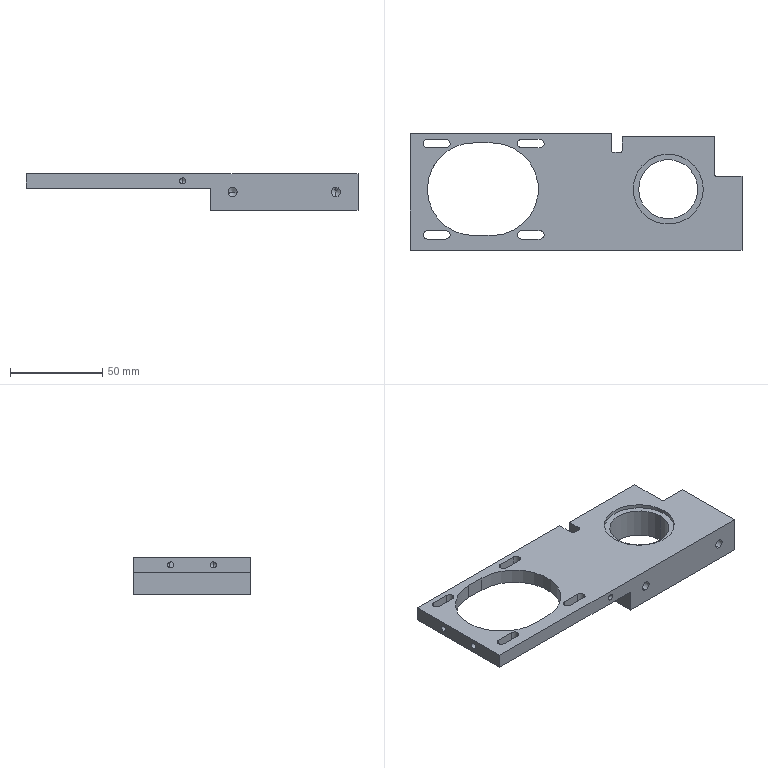Part | STEP file | 866-BDO024-95-05A | 1 solid | 85 faces | box 180 x 63 x 20 mm | volume 101274 mm3 | cylinder 42 | plane 26 | cone 17 | commonest cylinder face diameters 3.3 x14 4.5 x12 5 x4 38 x4 2 x3 50.2 x3